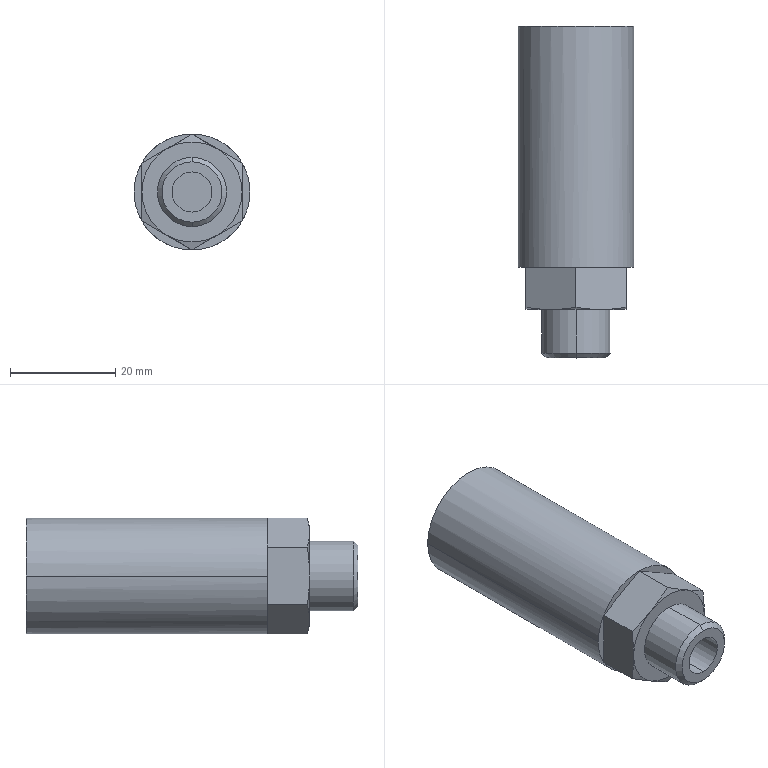Part | STEP file | 1 solid | 25 faces | box 22 x 63 x 22 mm | volume 20442 mm3 | plane 11 | cone 8 | cylinder 6 | commonest cylinder face diameters 7.6 x2 13.157 x2 22 x2